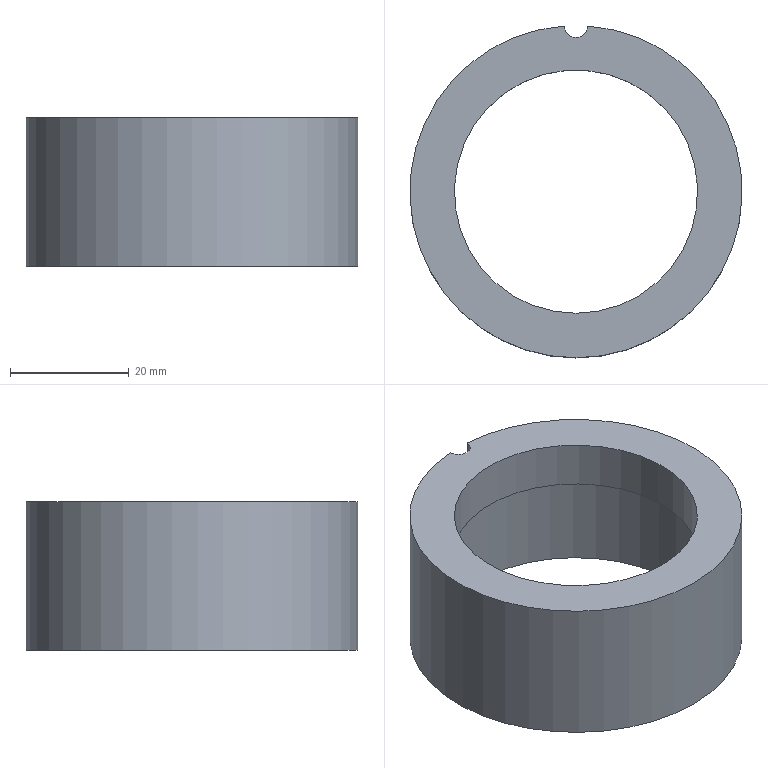Part | NX | features solid 2 | 1 solid | 7 faces | box 56 x 55.929 x 25 mm | volume 22606 mm3 | cylinder 4 | plane 3 | commonest cylinder face diameters 4 x1 41 x1 46 x1 56 x1
STEP:
#1=CARTESIAN_POINT('',(-781.999,-2.071,26.));
#2=VERTEX_POINT('',#1);
#3=CARTESIAN_POINT('',(-778.001,-2.071,26.));
#4=VERTEX_POINT('',#3);
#5=CARTESIAN_POINT('',(-780.,-30.,26.));
#6=DIRECTION('',(0.,0.,1.));
#7=DIRECTION('',(0.,-1.,0.));
#8=AXIS2_PLACEMENT_3D('',#5,#6,#7);
#9=CIRCLE('',#8,28.);
#10=EDGE_CURVE('',#2,#4,#9,.T.);
#11=ORIENTED_EDGE('',*,*,#10,.F.);
#12=CARTESIAN_POINT('',(-780.,-2.,26.));
#13=DIRECTION('',(0.,0.,1.));
#14=DIRECTION('',(0.,-1.,0.));
#15=AXIS2_PLACEMENT_3D('',#12,#13,#14);
#16=CIRCLE('',#15,2.);
#17=EDGE_CURVE('',#2,#4,#16,.T.);
#18=ORIENTED_EDGE('',*,*,#17,.T.);
#19=EDGE_LOOP('',(#11,#18));
#20=FACE_BOUND('',#19,.T.);
#21=CARTESIAN_POINT('',(-780.,-53.,26.));
#22=VERTEX_POINT('',#21);
#23=CARTESIAN_POINT('',(-780.,-30.,26.));
#24=DIRECTION('',(0.,0.,1.));
#25=DIRECTION('',(0.,-1.,0.));
#26=AXIS2_PLACEMENT_3D('',#23,#24,#25);
#27=CIRCLE('',#26,23.);
#28=EDGE_CURVE('',#22,#22,#27,.F.);
#29=ORIENTED_EDGE('',*,*,#28,.F.);
#30=EDGE_LOOP('',(#29));
#31=FACE_BOUND('',#30,.T.);
#32=CARTESIAN_POINT('',(-780.,-30.,26.));
#33=DIRECTION('',(0.,0.,1.));
#34=DIRECTION('',(0.,-1.,0.));
#35=AXIS2_PLACEMENT_3D('',#32,#33,#34);
#36=PLANE('',#35);
#37=ADVANCED_FACE('',(#20,#31),#36,.F.);
#38=CARTESIAN_POINT('',(-778.001,-2.071,51.));
#39=VERTEX_POINT('',#38);
#40=CARTESIAN_POINT('',(-781.999,-2.071,51.));
#41=VERTEX_POINT('',#40);
#42=CARTESIAN_POINT('',(-780.,-2.,51.));
#43=DIRECTION('',(0.,0.,-1.));
#44=DIRECTION('',(0.,1.,0.));
#45=AXIS2_PLACEMENT_3D('',#42,#43,#44);
#46=CIRCLE('',#45,2.);
#47=EDGE_CURVE('',#39,#41,#46,.T.);
#48=ORIENTED_EDGE('',*,*,#47,.T.);
#49=CARTESIAN_POINT('',(-780.,-30.,51.));
#50=DIRECTION('',(0.,0.,1.));
#51=DIRECTION('',(0.,-1.,0.));
#52=AXIS2_PLACEMENT_3D('',#49,#50,#51);
#53=CIRCLE('',#52,28.);
#54=EDGE_CURVE('',#41,#39,#53,.T.);
#55=ORIENTED_EDGE('',*,*,#54,.T.);
#56=EDGE_LOOP('',(#48,#55));
#57=FACE_BOUND('',#56,.T.);
#58=CARTESIAN_POINT('',(-780.,-50.5,51.));
#59=VERTEX_POINT('',#58);
#60=CARTESIAN_POINT('',(-780.,-30.,51.));
#61=DIRECTION('',(0.,0.,1.));
#62=DIRECTION('',(0.,-1.,0.));
#63=AXIS2_PLACEMENT_3D('',#60,#61,#62);
#64=CIRCLE('',#63,20.5);
#65=EDGE_CURVE('',#59,#59,#64,.F.);
#66=ORIENTED_EDGE('',*,*,#65,.T.);
#67=EDGE_LOOP('',(#66));
#68=FACE_BOUND('',#67,.T.);
#69=CARTESIAN_POINT('',(-780.,-30.,51.));
#70=DIRECTION('',(0.,0.,1.));
#71=DIRECTION('',(0.,-1.,0.));
#72=AXIS2_PLACEMENT_3D('',#69,#70,#71);
#73=PLANE('',#72);
#74=ADVANCED_FACE('',(#57,#68),#73,.T.);
#75=ORIENTED_EDGE('',*,*,#10,.T.);
#76=CARTESIAN_POINT('',(-778.001,-2.071,38.5));
#77=DIRECTION('',(0.,0.,-1.));
#78=VECTOR('',#77,1000.);
#79=LINE('',#76,#78);
#80=EDGE_CURVE('',#4,#39,#79,.F.);
#81=ORIENTED_EDGE('',*,*,#80,.T.);
#82=ORIENTED_EDGE('',*,*,#54,.F.);
#83=CARTESIAN_POINT('',(-781.999,-2.071,38.5));
#84=DIRECTION('',(0.,0.,-1.));
#85=VECTOR('',#84,1000.);
#86=LINE('',#83,#85);
#87=EDGE_CURVE('',#41,#2,#86,.T.);
#88=ORIENTED_EDGE('',*,*,#87,.T.);
#89=EDGE_LOOP('',(#75,#81,#82,#88));
#90=FACE_BOUND('',#89,.T.);
#91=CARTESIAN_POINT('',(-780.,-30.,51.));
#92=DIRECTION('',(0.,0.,-1.));
#93=DIRECTION('',(0.,1.,0.));
#94=AXIS2_PLACEMENT_3D('',#91,#92,#93);
#95=CYLINDRICAL_SURFACE('',#94,28.);
#96=ADVANCED_FACE('',(#90),#95,.T.);
#97=CARTESIAN_POINT('',(-780.,-50.5,43.));
#98=VERTEX_POINT('',#97);
#99=CARTESIAN_POINT('',(-780.,-30.,43.));
#100=DIRECTION('',(0.,0.,1.));
#101=DIRECTION('',(0.,-1.,0.));
#102=AXIS2_PLACEMENT_3D('',#99,#100,#101);
#103=CIRCLE('',#102,20.5);
#104=EDGE_CURVE('',#98,#98,#103,.T.);
#105=ORIENTED_EDGE('',*,*,#104,.F.);
#106=EDGE_LOOP('',(#105));
#107=FACE_BOUND('',#106,.T.);
#108=ORIENTED_EDGE('',*,*,#65,.F.);
#109=EDGE_LOOP('',(#108));
#110=FACE_BOUND('',#109,.T.);
#111=CARTESIAN_POINT('',(-780.,-30.,26.));
#112=DIRECTION('',(0.,0.,1.));
#113=DIRECTION('',(0.,-1.,0.));
#114=AXIS2_PLACEMENT_3D('',#111,#112,#113);
#115=CYLINDRICAL_SURFACE('',#114,20.5);
#116=ADVANCED_FACE('',(#107,#110),#115,.F.);
#117=CARTESIAN_POINT('',(-780.,-53.,43.));
#118=VERTEX_POINT('',#117);
#119=CARTESIAN_POINT('',(-780.,-30.,43.));
#120=DIRECTION('',(0.,0.,1.));
#121=DIRECTION('',(0.,-1.,0.));
#122=AXIS2_PLACEMENT_3D('',#119,#120,#121);
#123=CIRCLE('',#122,23.);
#124=EDGE_CURVE('',#118,#118,#123,.T.);
#125=ORIENTED_EDGE('',*,*,#124,.T.);
#126=EDGE_LOOP('',(#125));
#127=FACE_BOUND('',#126,.T.);
#128=ORIENTED_EDGE('',*,*,#28,.T.);
#129=EDGE_LOOP('',(#128));
#130=FACE_BOUND('',#129,.T.);
#131=CARTESIAN_POINT('',(-780.,-30.,43.));
#132=DIRECTION('',(0.,0.,-1.));
#133=DIRECTION('',(0.,1.,0.));
#134=AXIS2_PLACEMENT_3D('',#131,#132,#133);
#135=CYLINDRICAL_SURFACE('',#134,23.);
#136=ADVANCED_FACE('',(#127,#130),#135,.F.);
#137=ORIENTED_EDGE('',*,*,#104,.T.);
#138=EDGE_LOOP('',(#137));
#139=FACE_BOUND('',#138,.T.);
#140=ORIENTED_EDGE('',*,*,#124,.F.);
#141=EDGE_LOOP('',(#140));
#142=FACE_BOUND('',#141,.T.);
#143=CARTESIAN_POINT('',(-780.,-30.,43.));
#144=DIRECTION('',(0.,0.,1.));
#145=DIRECTION('',(0.,-1.,0.));
#146=AXIS2_PLACEMENT_3D('',#143,#144,#145);
#147=PLANE('',#146);
#148=ADVANCED_FACE('',(#139,#142),#147,.F.);
#149=ORIENTED_EDGE('',*,*,#17,.F.);
#150=ORIENTED_EDGE('',*,*,#87,.F.);
#151=ORIENTED_EDGE('',*,*,#47,.F.);
#152=ORIENTED_EDGE('',*,*,#80,.F.);
#153=EDGE_LOOP('',(#149,#150,#151,#152));
#154=FACE_BOUND('',#153,.T.);
#155=CARTESIAN_POINT('',(-780.,-2.,51.));
#156=DIRECTION('',(0.,0.,-1.));
#157=DIRECTION('',(0.,1.,0.));
#158=AXIS2_PLACEMENT_3D('',#155,#156,#157);
#159=CYLINDRICAL_SURFACE('',#158,2.);
#160=ADVANCED_FACE('',(#154),#159,.F.);
#161=CLOSED_SHELL('',(#37,#74,#96,#116,#136,#148,#160));
#162=MANIFOLD_SOLID_BREP('',#161);
#163=(LENGTH_UNIT()NAMED_UNIT(*)SI_UNIT(.MILLI.,.METRE.));
#164=UNCERTAINTY_MEASURE_WITH_UNIT(LENGTH_MEASURE(0.00001),#163,'','');
#165=(NAMED_UNIT(*)PLANE_ANGLE_UNIT()SI_UNIT($,.RADIAN.));
#166=(NAMED_UNIT(*)SI_UNIT($,.STERADIAN.)SOLID_ANGLE_UNIT());
#167=(GEOMETRIC_REPRESENTATION_CONTEXT(3)GLOBAL_UNCERTAINTY_ASSIGNED_CONTEXT((#164))GLOBAL_UNIT_ASSIGNED_CONTEXT((#163,#165,#166))REPRESENTATION_CONTEXT('',''));
#168=ADVANCED_BREP_SHAPE_REPRESENTATION('',(#162),#167);